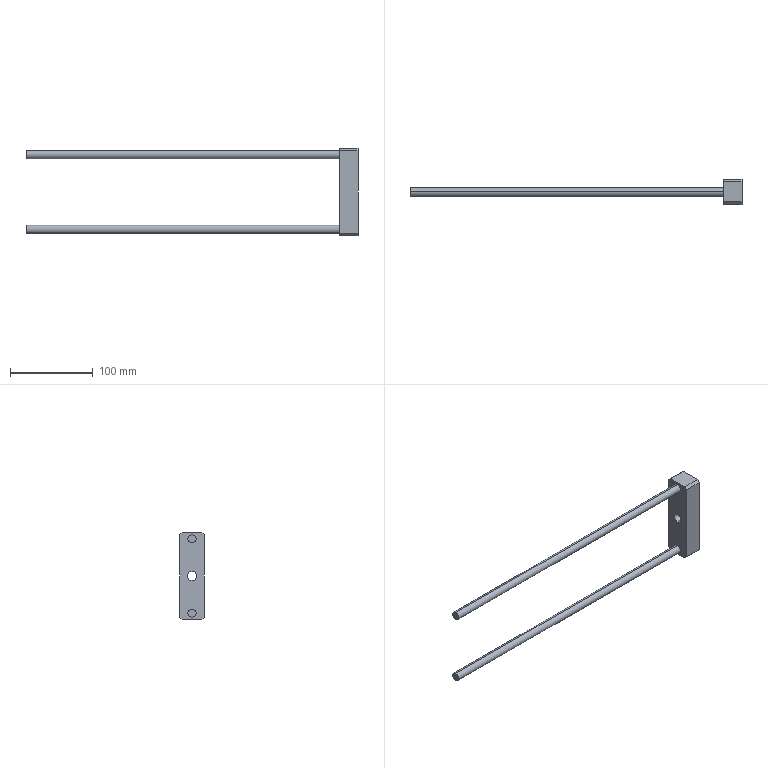Part | STEP file | Guide wheel mechanism revised.sldasm-Part-470 | 1 solid | 69 faces | box 400.5 x 30 x 105 mm | volume 119051 mm3 | cone 32 | cylinder 24 | plane 13 | commonest cylinder face diameters 4.134 x16 10 x4 11 x2 26 x2